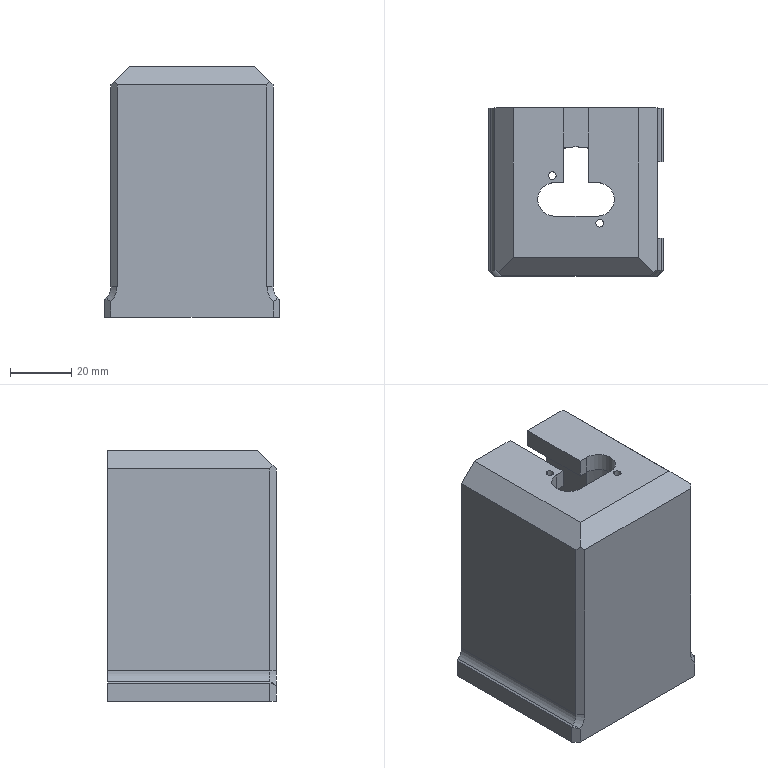Part | 1 solid | 111 faces | box 57 x 55 x 82 mm | volume 106355 mm3 | cylinder 50 | plane 43 | cone 18 | commonest cylinder face diameters 2.5 x16 3 x8 3.3 x8 11 x6 4 x4 7 x3